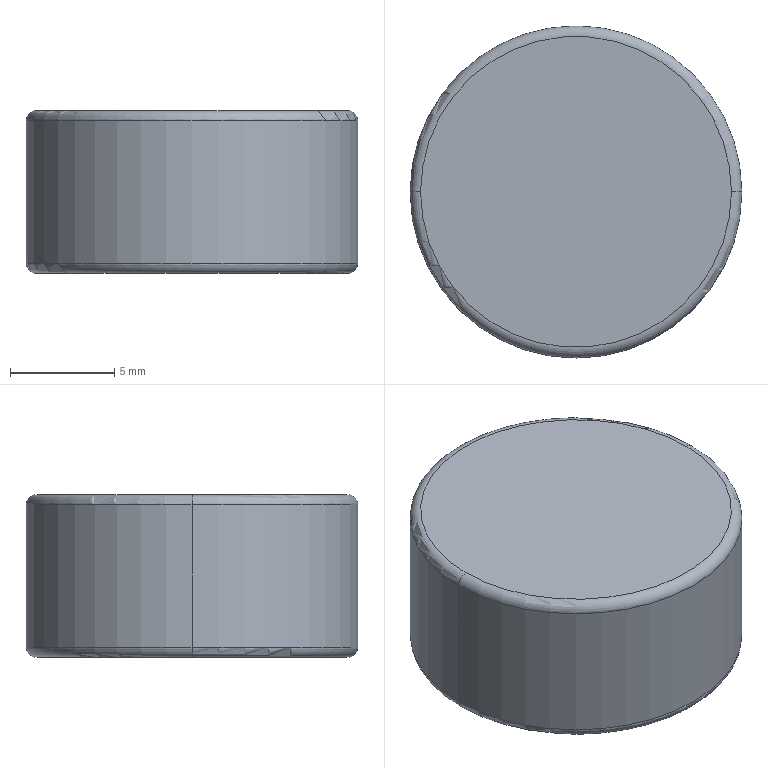Part | STEP file | RS40-AS-2LSR-T-266L-JR-Part-201-1 | 1 solid | 8 faces | box 15.88 x 15.88 x 7.8 mm | volume 1540 mm3 | torus 4 | cylinder 2 | plane 2 | commonest cylinder face diameters 15.88 x2
STEP:
#1=CARTESIAN_POINT('',(1565.7,77.06,7.3));
#2=VERTEX_POINT('',#1);
#3=CARTESIAN_POINT('',(1581.58,77.06,7.3));
#4=VERTEX_POINT('',#3);
#5=CARTESIAN_POINT('',(1573.64,77.06,7.3));
#6=DIRECTION('',(0.,0.,-1.));
#7=DIRECTION('',(1.,0.,0.));
#8=AXIS2_PLACEMENT_3D('',#5,#6,#7);
#9=CIRCLE('',#8,7.94);
#10=EDGE_CURVE('',#2,#4,#9,.T.);
#11=ORIENTED_EDGE('',*,*,#10,.F.);
#12=CARTESIAN_POINT('',(1566.2,77.06,7.8));
#13=VERTEX_POINT('',#12);
#14=CARTESIAN_POINT('',(1566.2,77.06,7.3));
#15=DIRECTION('',(0.,1.,0.));
#16=DIRECTION('',(-1.,0.,0.));
#17=AXIS2_PLACEMENT_3D('',#14,#15,#16);
#18=CIRCLE('',#17,0.5);
#19=EDGE_CURVE('',#2,#13,#18,.T.);
#20=ORIENTED_EDGE('',*,*,#19,.T.);
#21=CARTESIAN_POINT('',(1581.08,77.06,7.8));
#22=VERTEX_POINT('',#21);
#23=CARTESIAN_POINT('',(1573.64,77.06,7.8));
#24=DIRECTION('',(0.,0.,1.));
#25=DIRECTION('',(1.,0.,0.));
#26=AXIS2_PLACEMENT_3D('',#23,#24,#25);
#27=CIRCLE('',#26,7.44);
#28=EDGE_CURVE('',#22,#13,#27,.T.);
#29=ORIENTED_EDGE('',*,*,#28,.F.);
#30=CARTESIAN_POINT('',(1581.08,77.06,7.3));
#31=DIRECTION('',(0.,-1.,0.));
#32=DIRECTION('',(0.,0.,-1.));
#33=AXIS2_PLACEMENT_3D('',#30,#31,#32);
#34=CIRCLE('',#33,0.5);
#35=EDGE_CURVE('',#4,#22,#34,.T.);
#36=ORIENTED_EDGE('',*,*,#35,.F.);
#37=EDGE_LOOP('',(#11,#20,#29,#36));
#38=FACE_OUTER_BOUND('',#37,.T.);
#39=CARTESIAN_POINT('',(1573.64,77.06,7.3));
#40=DIRECTION('',(0.,0.,1.));
#41=DIRECTION('',(1.,0.,0.));
#42=AXIS2_PLACEMENT_3D('',#39,#40,#41);
#43=TOROIDAL_SURFACE('',#42,7.44,0.5);
#44=ADVANCED_FACE('',(#38),#43,.T.);
#45=CARTESIAN_POINT('',(1581.58,77.06,0.5));
#46=VERTEX_POINT('',#45);
#47=CARTESIAN_POINT('',(1565.7,77.06,0.5));
#48=VERTEX_POINT('',#47);
#49=CARTESIAN_POINT('',(1573.64,77.06,0.5));
#50=DIRECTION('',(0.,0.,1.));
#51=DIRECTION('',(1.,0.,0.));
#52=AXIS2_PLACEMENT_3D('',#49,#50,#51);
#53=CIRCLE('',#52,7.94);
#54=EDGE_CURVE('',#46,#48,#53,.T.);
#55=ORIENTED_EDGE('',*,*,#54,.F.);
#56=CARTESIAN_POINT('',(1581.077,77.06,0.));
#57=VERTEX_POINT('',#56);
#58=CARTESIAN_POINT('',(1581.077,77.06,0.5033));
#59=DIRECTION('',(0.,1.,0.));
#60=DIRECTION('',(-1.,0.,0.));
#61=AXIS2_PLACEMENT_3D('',#58,#59,#60);
#62=CIRCLE('',#61,0.5033);
#63=EDGE_CURVE('',#46,#57,#62,.T.);
#64=ORIENTED_EDGE('',*,*,#63,.T.);
#65=CARTESIAN_POINT('',(1566.203,77.06,0.));
#66=VERTEX_POINT('',#65);
#67=CARTESIAN_POINT('',(1573.64,77.06,0.));
#68=DIRECTION('',(0.,0.,-1.));
#69=DIRECTION('',(-1.,0.,0.));
#70=AXIS2_PLACEMENT_3D('',#67,#68,#69);
#71=CIRCLE('',#70,7.437);
#72=EDGE_CURVE('',#66,#57,#71,.T.);
#73=ORIENTED_EDGE('',*,*,#72,.F.);
#74=CARTESIAN_POINT('',(1566.203,77.06,0.5033));
#75=DIRECTION('',(0.,-1.,0.));
#76=DIRECTION('',(0.,0.,-1.));
#77=AXIS2_PLACEMENT_3D('',#74,#75,#76);
#78=CIRCLE('',#77,0.5033);
#79=EDGE_CURVE('',#48,#66,#78,.T.);
#80=ORIENTED_EDGE('',*,*,#79,.F.);
#81=EDGE_LOOP('',(#55,#64,#73,#80));
#82=FACE_OUTER_BOUND('',#81,.T.);
#83=CARTESIAN_POINT('',(1573.64,77.06,0.5033));
#84=DIRECTION('',(0.,0.,-1.));
#85=DIRECTION('',(-1.,0.,0.));
#86=AXIS2_PLACEMENT_3D('',#83,#84,#85);
#87=TOROIDAL_SURFACE('',#86,7.437,0.5033);
#88=ADVANCED_FACE('',(#82),#87,.T.);
#89=ORIENTED_EDGE('',*,*,#54,.T.);
#90=CARTESIAN_POINT('',(1565.7,77.06,-2.725));
#91=DIRECTION('',(0.,0.,1.));
#92=VECTOR('',#91,1000.);
#93=LINE('',#90,#92);
#94=EDGE_CURVE('',#48,#2,#93,.T.);
#95=ORIENTED_EDGE('',*,*,#94,.T.);
#96=ORIENTED_EDGE('',*,*,#10,.T.);
#97=CARTESIAN_POINT('',(1581.58,77.06,-2.725));
#98=DIRECTION('',(0.,0.,1.));
#99=VECTOR('',#98,1000.);
#100=LINE('',#97,#99);
#101=EDGE_CURVE('',#46,#4,#100,.T.);
#102=ORIENTED_EDGE('',*,*,#101,.F.);
#103=EDGE_LOOP('',(#89,#95,#96,#102));
#104=FACE_OUTER_BOUND('',#103,.T.);
#105=CARTESIAN_POINT('',(1573.64,77.06,-2.725));
#106=DIRECTION('',(0.,0.,1.));
#107=DIRECTION('',(1.,0.,0.));
#108=AXIS2_PLACEMENT_3D('',#105,#106,#107);
#109=CYLINDRICAL_SURFACE('',#108,7.94);
#110=ADVANCED_FACE('',(#104),#109,.T.);
#111=ORIENTED_EDGE('',*,*,#28,.T.);
#112=CARTESIAN_POINT('',(1573.64,77.06,7.8));
#113=DIRECTION('',(0.,0.,1.));
#114=DIRECTION('',(1.,0.,0.));
#115=AXIS2_PLACEMENT_3D('',#112,#113,#114);
#116=CIRCLE('',#115,7.44);
#117=EDGE_CURVE('',#13,#22,#116,.T.);
#118=ORIENTED_EDGE('',*,*,#117,.T.);
#119=EDGE_LOOP('',(#111,#118));
#120=FACE_OUTER_BOUND('',#119,.T.);
#121=CARTESIAN_POINT('',(1573.64,77.06,7.8));
#122=DIRECTION('',(0.,0.,1.));
#123=DIRECTION('',(1.,0.,0.));
#124=AXIS2_PLACEMENT_3D('',#121,#122,#123);
#125=PLANE('',#124);
#126=ADVANCED_FACE('',(#120),#125,.T.);
#127=ORIENTED_EDGE('',*,*,#94,.F.);
#128=CARTESIAN_POINT('',(1573.64,77.06,0.5));
#129=DIRECTION('',(0.,0.,1.));
#130=DIRECTION('',(1.,0.,0.));
#131=AXIS2_PLACEMENT_3D('',#128,#129,#130);
#132=CIRCLE('',#131,7.94);
#133=EDGE_CURVE('',#48,#46,#132,.T.);
#134=ORIENTED_EDGE('',*,*,#133,.T.);
#135=ORIENTED_EDGE('',*,*,#101,.T.);
#136=CARTESIAN_POINT('',(1573.64,77.06,7.3));
#137=DIRECTION('',(0.,0.,-1.));
#138=DIRECTION('',(1.,0.,0.));
#139=AXIS2_PLACEMENT_3D('',#136,#137,#138);
#140=CIRCLE('',#139,7.94);
#141=EDGE_CURVE('',#4,#2,#140,.T.);
#142=ORIENTED_EDGE('',*,*,#141,.T.);
#143=EDGE_LOOP('',(#127,#134,#135,#142));
#144=FACE_OUTER_BOUND('',#143,.T.);
#145=CARTESIAN_POINT('',(1573.64,77.06,-2.725));
#146=DIRECTION('',(0.,0.,1.));
#147=DIRECTION('',(1.,0.,0.));
#148=AXIS2_PLACEMENT_3D('',#145,#146,#147);
#149=CYLINDRICAL_SURFACE('',#148,7.94);
#150=ADVANCED_FACE('',(#144),#149,.T.);
#151=ORIENTED_EDGE('',*,*,#72,.T.);
#152=CARTESIAN_POINT('',(1573.64,77.06,0.));
#153=DIRECTION('',(0.,0.,-1.));
#154=DIRECTION('',(-1.,0.,0.));
#155=AXIS2_PLACEMENT_3D('',#152,#153,#154);
#156=CIRCLE('',#155,7.437);
#157=EDGE_CURVE('',#57,#66,#156,.T.);
#158=ORIENTED_EDGE('',*,*,#157,.T.);
#159=EDGE_LOOP('',(#151,#158));
#160=FACE_OUTER_BOUND('',#159,.T.);
#161=CARTESIAN_POINT('',(1565.703,77.06,0.));
#162=DIRECTION('',(0.,0.,-1.));
#163=DIRECTION('',(-1.,0.,0.));
#164=AXIS2_PLACEMENT_3D('',#161,#162,#163);
#165=PLANE('',#164);
#166=ADVANCED_FACE('',(#160),#165,.T.);
#167=ORIENTED_EDGE('',*,*,#63,.F.);
#168=ORIENTED_EDGE('',*,*,#133,.F.);
#169=ORIENTED_EDGE('',*,*,#79,.T.);
#170=ORIENTED_EDGE('',*,*,#157,.F.);
#171=EDGE_LOOP('',(#167,#168,#169,#170));
#172=FACE_OUTER_BOUND('',#171,.T.);
#173=CARTESIAN_POINT('',(1573.64,77.06,0.5033));
#174=DIRECTION('',(0.,0.,-1.));
#175=DIRECTION('',(-1.,0.,0.));
#176=AXIS2_PLACEMENT_3D('',#173,#174,#175);
#177=TOROIDAL_SURFACE('',#176,7.437,0.5033);
#178=ADVANCED_FACE('',(#172),#177,.T.);
#179=ORIENTED_EDGE('',*,*,#19,.F.);
#180=ORIENTED_EDGE('',*,*,#141,.F.);
#181=ORIENTED_EDGE('',*,*,#35,.T.);
#182=ORIENTED_EDGE('',*,*,#117,.F.);
#183=EDGE_LOOP('',(#179,#180,#181,#182));
#184=FACE_OUTER_BOUND('',#183,.T.);
#185=CARTESIAN_POINT('',(1573.64,77.06,7.3));
#186=DIRECTION('',(0.,0.,1.));
#187=DIRECTION('',(1.,0.,0.));
#188=AXIS2_PLACEMENT_3D('',#185,#186,#187);
#189=TOROIDAL_SURFACE('',#188,7.44,0.5);
#190=ADVANCED_FACE('',(#184),#189,.T.);
#191=CLOSED_SHELL('',(#44,#88,#110,#126,#150,#166,#178,#190));
#192=MANIFOLD_SOLID_BREP('',#191);
#193=CARTESIAN_POINT('',(0.,0.,0.));
#194=DIRECTION('',(0.,0.,1.));
#195=DIRECTION('',(1.,0.,0.));
#196=AXIS2_PLACEMENT_3D('',#193,#194,#195);
#197=(LENGTH_UNIT()NAMED_UNIT(*)SI_UNIT(.MILLI.,.METRE.));
#198=UNCERTAINTY_MEASURE_WITH_UNIT(LENGTH_MEASURE(0.00001),#197,'','');
#199=(NAMED_UNIT(*)PLANE_ANGLE_UNIT()SI_UNIT($,.RADIAN.));
#200=(NAMED_UNIT(*)SI_UNIT($,.STERADIAN.)SOLID_ANGLE_UNIT());
#201=(GEOMETRIC_REPRESENTATION_CONTEXT(3)GLOBAL_UNCERTAINTY_ASSIGNED_CONTEXT((#198))GLOBAL_UNIT_ASSIGNED_CONTEXT((#197,#199,#200))REPRESENTATION_CONTEXT('',''));
#202=ADVANCED_BREP_SHAPE_REPRESENTATION('',(#192,#196),#201);